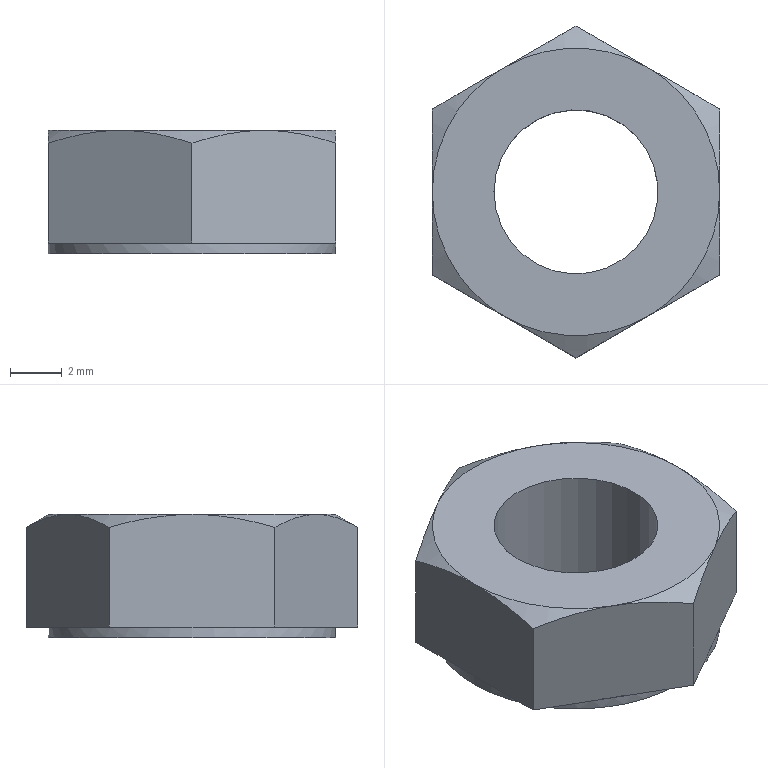Part | NX | features solid 2 | 1 solid | 22 faces | box 11.125 x 12.846 x 4.763 mm | volume 354.079 mm3 | plane 14 | cone 6 | cylinder 2 | commonest cylinder face diameters 6.35 x1 11.125 x1
STEP:
#1=CARTESIAN_POINT('',(2.781,4.817,4.763));
#2=VERTEX_POINT('',#1);
#3=CARTESIAN_POINT('',(0.,6.423,4.266));
#4=VERTEX_POINT('',#3);
#5=CARTESIAN_POINT('',(2.781,4.817,4.763));
#6=CARTESIAN_POINT('',(1.837,5.362,4.763));
#7=CARTESIAN_POINT('',(0.9077,5.899,4.568));
#8=CARTESIAN_POINT('',(0.,6.423,4.266));
#9=B_SPLINE_CURVE_WITH_KNOTS('',3,(#5,#6,#7,#8),.UNSPECIFIED.,.F.,.F.,(4,4),(0.00325,0.006487),.UNSPECIFIED.);
#10=EDGE_CURVE('',#2,#4,#9,.T.);
#11=ORIENTED_EDGE('',*,*,#10,.T.);
#12=CARTESIAN_POINT('',(-2.781,4.817,4.763));
#13=VERTEX_POINT('',#12);
#14=CARTESIAN_POINT('',(0.,6.423,4.266));
#15=CARTESIAN_POINT('',(-0.91,5.898,4.569));
#16=CARTESIAN_POINT('',(-1.834,5.365,4.763));
#17=CARTESIAN_POINT('',(-2.781,4.817,4.763));
#18=B_SPLINE_CURVE_WITH_KNOTS('',3,(#14,#15,#16,#17),.UNSPECIFIED.,.F.,.F.,(4,4),(0.000000238,0.00325),.UNSPECIFIED.);
#19=EDGE_CURVE('',#4,#13,#18,.T.);
#20=ORIENTED_EDGE('',*,*,#19,.T.);
#21=CARTESIAN_POINT('',(0.,0.,4.763));
#22=DIRECTION('',(0.,0.,-1.));
#23=DIRECTION('',(-1.,0.,0.));
#24=AXIS2_PLACEMENT_3D('',#21,#22,#23);
#25=CIRCLE('',#24,5.563);
#26=EDGE_CURVE('',#13,#2,#25,.T.);
#27=ORIENTED_EDGE('',*,*,#26,.T.);
#28=EDGE_LOOP('',(#11,#20,#27));
#29=FACE_BOUND('',#28,.T.);
#30=CARTESIAN_POINT('',(0.,0.,4.763));
#31=DIRECTION('',(0.,0.,-1.));
#32=DIRECTION('',(-1.,0.,0.));
#33=AXIS2_PLACEMENT_3D('',#30,#31,#32);
#34=CONICAL_SURFACE('',#33,5.563,1.047);
#35=ADVANCED_FACE('',(#29),#34,.T.);
#36=CARTESIAN_POINT('',(-5.563,0.,4.763));
#37=VERTEX_POINT('',#36);
#38=CARTESIAN_POINT('',(0.,0.,4.763));
#39=DIRECTION('',(0.,0.,-1.));
#40=DIRECTION('',(-1.,0.,0.));
#41=AXIS2_PLACEMENT_3D('',#38,#39,#40);
#42=CIRCLE('',#41,5.563);
#43=EDGE_CURVE('',#37,#13,#42,.T.);
#44=ORIENTED_EDGE('',*,*,#43,.T.);
#45=CARTESIAN_POINT('',(-5.563,3.212,4.266));
#46=VERTEX_POINT('',#45);
#47=CARTESIAN_POINT('',(-2.781,4.817,4.763));
#48=CARTESIAN_POINT('',(-3.725,4.272,4.763));
#49=CARTESIAN_POINT('',(-4.655,3.736,4.568));
#50=CARTESIAN_POINT('',(-5.563,3.212,4.266));
#51=B_SPLINE_CURVE_WITH_KNOTS('',3,(#47,#48,#49,#50),.UNSPECIFIED.,.F.,.F.,(4,4),(0.00325,0.006487),.UNSPECIFIED.);
#52=EDGE_CURVE('',#13,#46,#51,.T.);
#53=ORIENTED_EDGE('',*,*,#52,.T.);
#54=CARTESIAN_POINT('',(-5.563,0.,4.763));
#55=CARTESIAN_POINT('',(-5.563,1.087,4.763));
#56=CARTESIAN_POINT('',(-5.563,2.173,4.566));
#57=CARTESIAN_POINT('',(-5.563,3.212,4.266));
#58=B_SPLINE_CURVE_WITH_KNOTS('',3,(#54,#55,#56,#57),.UNSPECIFIED.,.F.,.F.,(4,4),(0.009152,0.01241),.UNSPECIFIED.);
#59=EDGE_CURVE('',#46,#37,#58,.F.);
#60=ORIENTED_EDGE('',*,*,#59,.T.);
#61=EDGE_LOOP('',(#44,#53,#60));
#62=FACE_BOUND('',#61,.T.);
#63=CARTESIAN_POINT('',(0.,0.,4.763));
#64=DIRECTION('',(0.,0.,-1.));
#65=DIRECTION('',(-1.,0.,0.));
#66=AXIS2_PLACEMENT_3D('',#63,#64,#65);
#67=CONICAL_SURFACE('',#66,5.563,1.047);
#68=ADVANCED_FACE('',(#62),#67,.T.);
#69=CARTESIAN_POINT('',(-2.781,-4.817,4.763));
#70=VERTEX_POINT('',#69);
#71=CARTESIAN_POINT('',(0.,0.,4.763));
#72=DIRECTION('',(0.,0.,-1.));
#73=DIRECTION('',(-1.,0.,0.));
#74=AXIS2_PLACEMENT_3D('',#71,#72,#73);
#75=CIRCLE('',#74,5.563);
#76=EDGE_CURVE('',#70,#37,#75,.T.);
#77=ORIENTED_EDGE('',*,*,#76,.T.);
#78=CARTESIAN_POINT('',(-5.563,-3.212,4.266));
#79=VERTEX_POINT('',#78);
#80=CARTESIAN_POINT('',(-5.563,-3.212,4.266));
#81=CARTESIAN_POINT('',(-5.563,-2.166,4.568));
#82=CARTESIAN_POINT('',(-5.563,-1.086,4.763));
#83=CARTESIAN_POINT('',(-5.563,0.,4.763));
#84=B_SPLINE_CURVE_WITH_KNOTS('',3,(#80,#81,#82,#83),.UNSPECIFIED.,.F.,.F.,(4,4),(0.005902,0.009152),.UNSPECIFIED.);
#85=EDGE_CURVE('',#37,#79,#84,.F.);
#86=ORIENTED_EDGE('',*,*,#85,.T.);
#87=CARTESIAN_POINT('',(-5.563,-3.212,4.266));
#88=CARTESIAN_POINT('',(-4.653,-3.737,4.569));
#89=CARTESIAN_POINT('',(-3.729,-4.27,4.763));
#90=CARTESIAN_POINT('',(-2.781,-4.817,4.763));
#91=B_SPLINE_CURVE_WITH_KNOTS('',3,(#87,#88,#89,#90),.UNSPECIFIED.,.F.,.F.,(4,4),(0.000000238,0.00325),.UNSPECIFIED.);
#92=EDGE_CURVE('',#79,#70,#91,.T.);
#93=ORIENTED_EDGE('',*,*,#92,.T.);
#94=EDGE_LOOP('',(#77,#86,#93));
#95=FACE_BOUND('',#94,.T.);
#96=CARTESIAN_POINT('',(0.,0.,4.763));
#97=DIRECTION('',(0.,0.,-1.));
#98=DIRECTION('',(-1.,0.,0.));
#99=AXIS2_PLACEMENT_3D('',#96,#97,#98);
#100=CONICAL_SURFACE('',#99,5.563,1.047);
#101=ADVANCED_FACE('',(#95),#100,.T.);
#102=CARTESIAN_POINT('',(2.781,-4.817,4.763));
#103=VERTEX_POINT('',#102);
#104=CARTESIAN_POINT('',(0.,0.,4.763));
#105=DIRECTION('',(0.,0.,-1.));
#106=DIRECTION('',(-1.,0.,0.));
#107=AXIS2_PLACEMENT_3D('',#104,#105,#106);
#108=CIRCLE('',#107,5.563);
#109=EDGE_CURVE('',#103,#70,#108,.T.);
#110=ORIENTED_EDGE('',*,*,#109,.T.);
#111=CARTESIAN_POINT('',(0.,-6.423,4.266));
#112=VERTEX_POINT('',#111);
#113=CARTESIAN_POINT('',(-2.781,-4.817,4.763));
#114=CARTESIAN_POINT('',(-1.837,-5.362,4.763));
#115=CARTESIAN_POINT('',(-0.9077,-5.899,4.568));
#116=CARTESIAN_POINT('',(0.,-6.423,4.266));
#117=B_SPLINE_CURVE_WITH_KNOTS('',3,(#113,#114,#115,#116),.UNSPECIFIED.,.F.,.F.,(4,4),(0.00325,0.006487),.UNSPECIFIED.);
#118=EDGE_CURVE('',#70,#112,#117,.T.);
#119=ORIENTED_EDGE('',*,*,#118,.T.);
#120=CARTESIAN_POINT('',(0.,-6.423,4.266));
#121=CARTESIAN_POINT('',(0.91,-5.898,4.569));
#122=CARTESIAN_POINT('',(1.834,-5.365,4.763));
#123=CARTESIAN_POINT('',(2.781,-4.817,4.763));
#124=B_SPLINE_CURVE_WITH_KNOTS('',3,(#120,#121,#122,#123),.UNSPECIFIED.,.F.,.F.,(4,4),(0.000000238,0.00325),.UNSPECIFIED.);
#125=EDGE_CURVE('',#112,#103,#124,.T.);
#126=ORIENTED_EDGE('',*,*,#125,.T.);
#127=EDGE_LOOP('',(#110,#119,#126));
#128=FACE_BOUND('',#127,.T.);
#129=CARTESIAN_POINT('',(0.,0.,4.763));
#130=DIRECTION('',(0.,0.,-1.));
#131=DIRECTION('',(-1.,0.,0.));
#132=AXIS2_PLACEMENT_3D('',#129,#130,#131);
#133=CONICAL_SURFACE('',#132,5.563,1.047);
#134=ADVANCED_FACE('',(#128),#133,.T.);
#135=CARTESIAN_POINT('',(5.563,0.,4.763));
#136=VERTEX_POINT('',#135);
#137=CARTESIAN_POINT('',(0.,0.,4.763));
#138=DIRECTION('',(0.,0.,-1.));
#139=DIRECTION('',(-1.,0.,0.));
#140=AXIS2_PLACEMENT_3D('',#137,#138,#139);
#141=CIRCLE('',#140,5.563);
#142=EDGE_CURVE('',#136,#103,#141,.T.);
#143=ORIENTED_EDGE('',*,*,#142,.T.);
#144=CARTESIAN_POINT('',(5.563,-3.212,4.266));
#145=VERTEX_POINT('',#144);
#146=CARTESIAN_POINT('',(2.781,-4.817,4.763));
#147=CARTESIAN_POINT('',(3.725,-4.272,4.763));
#148=CARTESIAN_POINT('',(4.655,-3.736,4.568));
#149=CARTESIAN_POINT('',(5.563,-3.212,4.266));
#150=B_SPLINE_CURVE_WITH_KNOTS('',3,(#146,#147,#148,#149),.UNSPECIFIED.,.F.,.F.,(4,4),(0.00325,0.006487),.UNSPECIFIED.);
#151=EDGE_CURVE('',#103,#145,#150,.T.);
#152=ORIENTED_EDGE('',*,*,#151,.T.);
#153=CARTESIAN_POINT('',(5.563,-3.212,4.266));
#154=CARTESIAN_POINT('',(5.563,-2.166,4.568));
#155=CARTESIAN_POINT('',(5.563,-1.086,4.763));
#156=CARTESIAN_POINT('',(5.563,0.,4.763));
#157=B_SPLINE_CURVE_WITH_KNOTS('',3,(#153,#154,#155,#156),.UNSPECIFIED.,.F.,.F.,(4,4),(0.005902,0.009152),.UNSPECIFIED.);
#158=EDGE_CURVE('',#145,#136,#157,.T.);
#159=ORIENTED_EDGE('',*,*,#158,.T.);
#160=EDGE_LOOP('',(#143,#152,#159));
#161=FACE_BOUND('',#160,.T.);
#162=CARTESIAN_POINT('',(0.,0.,4.763));
#163=DIRECTION('',(0.,0.,-1.));
#164=DIRECTION('',(-1.,0.,0.));
#165=AXIS2_PLACEMENT_3D('',#162,#163,#164);
#166=CONICAL_SURFACE('',#165,5.563,1.047);
#167=ADVANCED_FACE('',(#161),#166,.T.);
#168=CARTESIAN_POINT('',(0.,0.,4.763));
#169=DIRECTION('',(0.,0.,-1.));
#170=DIRECTION('',(-1.,0.,0.));
#171=AXIS2_PLACEMENT_3D('',#168,#169,#170);
#172=CIRCLE('',#171,5.563);
#173=EDGE_CURVE('',#2,#136,#172,.T.);
#174=ORIENTED_EDGE('',*,*,#173,.T.);
#175=CARTESIAN_POINT('',(5.563,3.212,4.266));
#176=VERTEX_POINT('',#175);
#177=CARTESIAN_POINT('',(5.563,0.,4.763));
#178=CARTESIAN_POINT('',(5.563,1.087,4.763));
#179=CARTESIAN_POINT('',(5.563,2.173,4.566));
#180=CARTESIAN_POINT('',(5.563,3.212,4.266));
#181=B_SPLINE_CURVE_WITH_KNOTS('',3,(#177,#178,#179,#180),.UNSPECIFIED.,.F.,.F.,(4,4),(0.009152,0.01241),.UNSPECIFIED.);
#182=EDGE_CURVE('',#136,#176,#181,.T.);
#183=ORIENTED_EDGE('',*,*,#182,.T.);
#184=CARTESIAN_POINT('',(5.563,3.212,4.266));
#185=CARTESIAN_POINT('',(4.653,3.737,4.569));
#186=CARTESIAN_POINT('',(3.729,4.27,4.763));
#187=CARTESIAN_POINT('',(2.781,4.817,4.763));
#188=B_SPLINE_CURVE_WITH_KNOTS('',3,(#184,#185,#186,#187),.UNSPECIFIED.,.F.,.F.,(4,4),(0.000000238,0.00325),.UNSPECIFIED.);
#189=EDGE_CURVE('',#176,#2,#188,.T.);
#190=ORIENTED_EDGE('',*,*,#189,.T.);
#191=EDGE_LOOP('',(#174,#183,#190));
#192=FACE_BOUND('',#191,.T.);
#193=CARTESIAN_POINT('',(0.,0.,4.763));
#194=DIRECTION('',(0.,0.,-1.));
#195=DIRECTION('',(-1.,0.,0.));
#196=AXIS2_PLACEMENT_3D('',#193,#194,#195);
#197=CONICAL_SURFACE('',#196,5.563,1.047);
#198=ADVANCED_FACE('',(#192),#197,.T.);
#199=CARTESIAN_POINT('',(2.781,-4.817,0.4064));
#200=VERTEX_POINT('',#199);
#201=CARTESIAN_POINT('',(0.,-6.423,0.4064));
#202=VERTEX_POINT('',#201);
#203=CARTESIAN_POINT('',(9.039,-1.204,0.4064));
#204=DIRECTION('',(-0.866,-0.5,0.));
#205=VECTOR('',#204,1000.);
#206=LINE('',#203,#205);
#207=EDGE_CURVE('',#200,#202,#206,.T.);
#208=ORIENTED_EDGE('',*,*,#207,.T.);
#209=CARTESIAN_POINT('',(-2.781,-4.817,0.4064));
#210=VERTEX_POINT('',#209);
#211=CARTESIAN_POINT('',(3.477,-8.43,0.4064));
#212=DIRECTION('',(-0.866,0.5,0.));
#213=VECTOR('',#212,1000.);
#214=LINE('',#211,#213);
#215=EDGE_CURVE('',#202,#210,#214,.T.);
#216=ORIENTED_EDGE('',*,*,#215,.T.);
#217=CARTESIAN_POINT('',(0.,0.,0.4064));
#218=DIRECTION('',(0.,0.,-1.));
#219=DIRECTION('',(-1.,0.,0.));
#220=AXIS2_PLACEMENT_3D('',#217,#218,#219);
#221=CIRCLE('',#220,5.563);
#222=EDGE_CURVE('',#200,#210,#221,.T.);
#223=ORIENTED_EDGE('',*,*,#222,.F.);
#224=EDGE_LOOP('',(#208,#216,#223));
#225=FACE_BOUND('',#224,.T.);
#226=CARTESIAN_POINT('',(8.344,0.,0.4064));
#227=DIRECTION('',(0.,0.,1.));
#228=DIRECTION('',(1.,0.,0.));
#229=AXIS2_PLACEMENT_3D('',#226,#227,#228);
#230=PLANE('',#229);
#231=ADVANCED_FACE('',(#225),#230,.F.);
#232=CARTESIAN_POINT('',(-5.563,0.,0.4064));
#233=VERTEX_POINT('',#232);
#234=CARTESIAN_POINT('',(0.,0.,0.4064));
#235=DIRECTION('',(0.,0.,-1.));
#236=DIRECTION('',(-1.,0.,0.));
#237=AXIS2_PLACEMENT_3D('',#234,#235,#236);
#238=CIRCLE('',#237,5.563);
#239=EDGE_CURVE('',#210,#233,#238,.T.);
#240=ORIENTED_EDGE('',*,*,#239,.F.);
#241=CARTESIAN_POINT('',(-5.563,-3.212,0.4064));
#242=VERTEX_POINT('',#241);
#243=CARTESIAN_POINT('',(3.477,-8.43,0.4064));
#244=DIRECTION('',(-0.866,0.5,0.));
#245=VECTOR('',#244,1000.);
#246=LINE('',#243,#245);
#247=EDGE_CURVE('',#210,#242,#246,.T.);
#248=ORIENTED_EDGE('',*,*,#247,.T.);
#249=CARTESIAN_POINT('',(-5.563,0.,0.4064));
#250=DIRECTION('',(0.,1.,0.));
#251=VECTOR('',#250,1000.);
#252=LINE('',#249,#251);
#253=EDGE_CURVE('',#242,#233,#252,.T.);
#254=ORIENTED_EDGE('',*,*,#253,.T.);
#255=EDGE_LOOP('',(#240,#248,#254));
#256=FACE_BOUND('',#255,.T.);
#257=CARTESIAN_POINT('',(8.344,0.,0.4064));
#258=DIRECTION('',(0.,0.,1.));
#259=DIRECTION('',(1.,0.,0.));
#260=AXIS2_PLACEMENT_3D('',#257,#258,#259);
#261=PLANE('',#260);
#262=ADVANCED_FACE('',(#256),#261,.F.);
#263=CARTESIAN_POINT('',(-2.781,4.817,0.4064));
#264=VERTEX_POINT('',#263);
#265=CARTESIAN_POINT('',(0.,0.,0.4064));
#266=DIRECTION('',(0.,0.,-1.));
#267=DIRECTION('',(-1.,0.,0.));
#268=AXIS2_PLACEMENT_3D('',#265,#266,#267);
#269=CIRCLE('',#268,5.563);
#270=EDGE_CURVE('',#233,#264,#269,.T.);
#271=ORIENTED_EDGE('',*,*,#270,.F.);
#272=CARTESIAN_POINT('',(-5.563,3.212,0.4064));
#273=VERTEX_POINT('',#272);
#274=CARTESIAN_POINT('',(-5.563,0.,0.4064));
#275=DIRECTION('',(0.,1.,0.));
#276=VECTOR('',#275,1000.);
#277=LINE('',#274,#276);
#278=EDGE_CURVE('',#233,#273,#277,.T.);
#279=ORIENTED_EDGE('',*,*,#278,.T.);
#280=CARTESIAN_POINT('',(3.477,8.43,0.4064));
#281=DIRECTION('',(0.866,0.5,0.));
#282=VECTOR('',#281,1000.);
#283=LINE('',#280,#282);
#284=EDGE_CURVE('',#273,#264,#283,.T.);
#285=ORIENTED_EDGE('',*,*,#284,.T.);
#286=EDGE_LOOP('',(#271,#279,#285));
#287=FACE_BOUND('',#286,.T.);
#288=CARTESIAN_POINT('',(8.344,0.,0.4064));
#289=DIRECTION('',(0.,0.,1.));
#290=DIRECTION('',(1.,0.,0.));
#291=AXIS2_PLACEMENT_3D('',#288,#289,#290);
#292=PLANE('',#291);
#293=ADVANCED_FACE('',(#287),#292,.F.);
#294=CARTESIAN_POINT('',(5.563,0.,0.4064));
#295=VERTEX_POINT('',#294);
#296=CARTESIAN_POINT('',(5.563,-3.212,0.4064));
#297=VERTEX_POINT('',#296);
#298=CARTESIAN_POINT('',(5.563,0.,0.4064));
#299=DIRECTION('',(0.,-1.,0.));
#300=VECTOR('',#299,1000.);
#301=LINE('',#298,#300);
#302=EDGE_CURVE('',#295,#297,#301,.T.);
#303=ORIENTED_EDGE('',*,*,#302,.T.);
#304=CARTESIAN_POINT('',(9.039,-1.204,0.4064));
#305=DIRECTION('',(-0.866,-0.5,0.));
#306=VECTOR('',#305,1000.);
#307=LINE('',#304,#306);
#308=EDGE_CURVE('',#297,#200,#307,.T.);
#309=ORIENTED_EDGE('',*,*,#308,.T.);
#310=CARTESIAN_POINT('',(0.,0.,0.4064));
#311=DIRECTION('',(0.,0.,-1.));
#312=DIRECTION('',(-1.,0.,0.));
#313=AXIS2_PLACEMENT_3D('',#310,#311,#312);
#314=CIRCLE('',#313,5.563);
#315=EDGE_CURVE('',#295,#200,#314,.T.);
#316=ORIENTED_EDGE('',*,*,#315,.F.);
#317=EDGE_LOOP('',(#303,#309,#316));
#318=FACE_BOUND('',#317,.T.);
#319=CARTESIAN_POINT('',(8.344,0.,0.4064));
#320=DIRECTION('',(0.,0.,1.));
#321=DIRECTION('',(1.,0.,0.));
#322=AXIS2_PLACEMENT_3D('',#319,#320,#321);
#323=PLANE('',#322);
#324=ADVANCED_FACE('',(#318),#323,.F.);
#325=CARTESIAN_POINT('',(2.781,4.817,0.4064));
#326=VERTEX_POINT('',#325);
#327=CARTESIAN_POINT('',(0.,0.,0.4064));
#328=DIRECTION('',(0.,0.,-1.));
#329=DIRECTION('',(-1.,0.,0.));
#330=AXIS2_PLACEMENT_3D('',#327,#328,#329);
#331=CIRCLE('',#330,5.563);
#332=EDGE_CURVE('',#264,#326,#331,.T.);
#333=ORIENTED_EDGE('',*,*,#332,.F.);
#334=CARTESIAN_POINT('',(0.,6.423,0.4064));
#335=VERTEX_POINT('',#334);
#336=CARTESIAN_POINT('',(3.477,8.43,0.4064));
#337=DIRECTION('',(0.866,0.5,0.));
#338=VECTOR('',#337,1000.);
#339=LINE('',#336,#338);
#340=EDGE_CURVE('',#264,#335,#339,.T.);
#341=ORIENTED_EDGE('',*,*,#340,.T.);
#342=CARTESIAN_POINT('',(9.039,1.204,0.4064));
#343=DIRECTION('',(0.866,-0.5,0.));
#344=VECTOR('',#343,1000.);
#345=LINE('',#342,#344);
#346=EDGE_CURVE('',#335,#326,#345,.T.);
#347=ORIENTED_EDGE('',*,*,#346,.T.);
#348=EDGE_LOOP('',(#333,#341,#347));
#349=FACE_BOUND('',#348,.T.);
#350=CARTESIAN_POINT('',(8.344,0.,0.4064));
#351=DIRECTION('',(0.,0.,1.));
#352=DIRECTION('',(1.,0.,0.));
#353=AXIS2_PLACEMENT_3D('',#350,#351,#352);
#354=PLANE('',#353);
#355=ADVANCED_FACE('',(#349),#354,.F.);
#356=CARTESIAN_POINT('',(5.563,3.212,0.4064));
#357=VERTEX_POINT('',#356);
#358=CARTESIAN_POINT('',(9.039,1.204,0.4064));
#359=DIRECTION('',(0.866,-0.5,0.));
#360=VECTOR('',#359,1000.);
#361=LINE('',#358,#360);
#362=EDGE_CURVE('',#326,#357,#361,.T.);
#363=ORIENTED_EDGE('',*,*,#362,.T.);
#364=CARTESIAN_POINT('',(5.563,0.,0.4064));
#365=DIRECTION('',(0.,-1.,0.));
#366=VECTOR('',#365,1000.);
#367=LINE('',#364,#366);
#368=EDGE_CURVE('',#357,#295,#367,.T.);
#369=ORIENTED_EDGE('',*,*,#368,.T.);
#370=CARTESIAN_POINT('',(0.,0.,0.4064));
#371=DIRECTION('',(0.,0.,-1.));
#372=DIRECTION('',(-1.,0.,0.));
#373=AXIS2_PLACEMENT_3D('',#370,#371,#372);
#374=CIRCLE('',#373,5.563);
#375=EDGE_CURVE('',#326,#295,#374,.T.);
#376=ORIENTED_EDGE('',*,*,#375,.F.);
#377=EDGE_LOOP('',(#363,#369,#376));
#378=FACE_BOUND('',#377,.T.);
#379=CARTESIAN_POINT('',(8.344,0.,0.4064));
#380=DIRECTION('',(0.,0.,1.));
#381=DIRECTION('',(1.,0.,0.));
#382=AXIS2_PLACEMENT_3D('',#379,#380,#381);
#383=PLANE('',#382);
#384=ADVANCED_FACE('',(#378),#383,.F.);
#385=ORIENTED_EDGE('',*,*,#43,.F.);
#386=ORIENTED_EDGE('',*,*,#76,.F.);
#387=ORIENTED_EDGE('',*,*,#109,.F.);
#388=ORIENTED_EDGE('',*,*,#142,.F.);
#389=ORIENTED_EDGE('',*,*,#173,.F.);
#390=ORIENTED_EDGE('',*,*,#26,.F.);
#391=EDGE_LOOP('',(#385,#386,#387,#388,#389,#390));
#392=FACE_BOUND('',#391,.T.);
#393=CARTESIAN_POINT('',(-3.175,0.,4.763));
#394=VERTEX_POINT('',#393);
#395=CARTESIAN_POINT('',(0.,0.,4.763));
#396=DIRECTION('',(0.,0.,-1.));
#397=DIRECTION('',(-1.,0.,0.));
#398=AXIS2_PLACEMENT_3D('',#395,#396,#397);
#399=CIRCLE('',#398,3.175);
#400=EDGE_CURVE('',#394,#394,#399,.T.);
#401=ORIENTED_EDGE('',*,*,#400,.T.);
#402=EDGE_LOOP('',(#401));
#403=FACE_BOUND('',#402,.T.);
#404=CARTESIAN_POINT('',(3.175,0.,4.763));
#405=DIRECTION('',(0.,0.,-1.));
#406=DIRECTION('',(-1.,0.,0.));
#407=AXIS2_PLACEMENT_3D('',#404,#405,#406);
#408=PLANE('',#407);
#409=ADVANCED_FACE('',(#392,#403),#408,.F.);
#410=CARTESIAN_POINT('',(-5.563,0.,0.));
#411=VERTEX_POINT('',#410);
#412=CARTESIAN_POINT('',(0.,0.,0.));
#413=DIRECTION('',(0.,0.,-1.));
#414=DIRECTION('',(-1.,0.,0.));
#415=AXIS2_PLACEMENT_3D('',#412,#413,#414);
#416=CIRCLE('',#415,5.563);
#417=EDGE_CURVE('',#411,#411,#416,.T.);
#418=ORIENTED_EDGE('',*,*,#417,.F.);
#419=EDGE_LOOP('',(#418));
#420=FACE_BOUND('',#419,.T.);
#421=ORIENTED_EDGE('',*,*,#270,.T.);
#422=ORIENTED_EDGE('',*,*,#332,.T.);
#423=ORIENTED_EDGE('',*,*,#375,.T.);
#424=ORIENTED_EDGE('',*,*,#315,.T.);
#425=ORIENTED_EDGE('',*,*,#222,.T.);
#426=ORIENTED_EDGE('',*,*,#239,.T.);
#427=EDGE_LOOP('',(#421,#422,#423,#424,#425,#426));
#428=FACE_BOUND('',#427,.T.);
#429=CARTESIAN_POINT('',(0.,0.,0.));
#430=DIRECTION('',(0.,0.,-1.));
#431=DIRECTION('',(-1.,0.,0.));
#432=AXIS2_PLACEMENT_3D('',#429,#430,#431);
#433=CYLINDRICAL_SURFACE('',#432,5.563);
#434=ADVANCED_FACE('',(#420,#428),#433,.T.);
#435=CARTESIAN_POINT('',(-3.175,0.,0.));
#436=VERTEX_POINT('',#435);
#437=CARTESIAN_POINT('',(0.,0.,0.));
#438=DIRECTION('',(0.,0.,-1.));
#439=DIRECTION('',(-1.,0.,0.));
#440=AXIS2_PLACEMENT_3D('',#437,#438,#439);
#441=CIRCLE('',#440,3.175);
#442=EDGE_CURVE('',#436,#436,#441,.T.);
#443=ORIENTED_EDGE('',*,*,#442,.F.);
#444=EDGE_LOOP('',(#443));
#445=FACE_BOUND('',#444,.T.);
#446=ORIENTED_EDGE('',*,*,#417,.T.);
#447=EDGE_LOOP('',(#446));
#448=FACE_BOUND('',#447,.T.);
#449=CARTESIAN_POINT('',(5.563,0.,0.));
#450=DIRECTION('',(0.,0.,1.));
#451=DIRECTION('',(1.,0.,0.));
#452=AXIS2_PLACEMENT_3D('',#449,#450,#451);
#453=PLANE('',#452);
#454=ADVANCED_FACE('',(#445,#448),#453,.F.);
#455=ORIENTED_EDGE('',*,*,#400,.F.);
#456=EDGE_LOOP('',(#455));
#457=FACE_BOUND('',#456,.T.);
#458=ORIENTED_EDGE('',*,*,#442,.T.);
#459=EDGE_LOOP('',(#458));
#460=FACE_BOUND('',#459,.T.);
#461=CARTESIAN_POINT('',(0.,0.,0.));
#462=DIRECTION('',(0.,0.,-1.));
#463=DIRECTION('',(-1.,0.,0.));
#464=AXIS2_PLACEMENT_3D('',#461,#462,#463);
#465=CYLINDRICAL_SURFACE('',#464,3.175);
#466=ADVANCED_FACE('',(#457,#460),#465,.F.);
#467=ORIENTED_EDGE('',*,*,#19,.F.);
#468=CARTESIAN_POINT('',(0.,6.423,5.239));
#469=DIRECTION('',(0.,0.,-1.));
#470=VECTOR('',#469,1000.);
#471=LINE('',#468,#470);
#472=EDGE_CURVE('',#4,#335,#471,.T.);
#473=ORIENTED_EDGE('',*,*,#472,.T.);
#474=ORIENTED_EDGE('',*,*,#340,.F.);
#475=ORIENTED_EDGE('',*,*,#284,.F.);
#476=CARTESIAN_POINT('',(-5.563,3.212,5.239));
#477=DIRECTION('',(0.,0.,-1.));
#478=VECTOR('',#477,1000.);
#479=LINE('',#476,#478);
#480=EDGE_CURVE('',#46,#273,#479,.T.);
#481=ORIENTED_EDGE('',*,*,#480,.F.);
#482=ORIENTED_EDGE('',*,*,#52,.F.);
#483=EDGE_LOOP('',(#467,#473,#474,#475,#481,#482));
#484=FACE_BOUND('',#483,.T.);
#485=CARTESIAN_POINT('',(0.,6.423,5.239));
#486=DIRECTION('',(0.5,-0.866,0.));
#487=DIRECTION('',(0.866,0.5,0.));
#488=AXIS2_PLACEMENT_3D('',#485,#486,#487);
#489=PLANE('',#488);
#490=ADVANCED_FACE('',(#484),#489,.F.);
#491=ORIENTED_EDGE('',*,*,#59,.F.);
#492=ORIENTED_EDGE('',*,*,#480,.T.);
#493=ORIENTED_EDGE('',*,*,#278,.F.);
#494=ORIENTED_EDGE('',*,*,#253,.F.);
#495=CARTESIAN_POINT('',(-5.563,-3.212,5.239));
#496=DIRECTION('',(0.,0.,-1.));
#497=VECTOR('',#496,1000.);
#498=LINE('',#495,#497);
#499=EDGE_CURVE('',#79,#242,#498,.T.);
#500=ORIENTED_EDGE('',*,*,#499,.F.);
#501=ORIENTED_EDGE('',*,*,#85,.F.);
#502=EDGE_LOOP('',(#491,#492,#493,#494,#500,#501));
#503=FACE_BOUND('',#502,.T.);
#504=CARTESIAN_POINT('',(-5.563,3.212,5.239));
#505=DIRECTION('',(1.,0.,0.));
#506=DIRECTION('',(0.,1.,0.));
#507=AXIS2_PLACEMENT_3D('',#504,#505,#506);
#508=PLANE('',#507);
#509=ADVANCED_FACE('',(#503),#508,.F.);
#510=ORIENTED_EDGE('',*,*,#92,.F.);
#511=ORIENTED_EDGE('',*,*,#499,.T.);
#512=ORIENTED_EDGE('',*,*,#247,.F.);
#513=ORIENTED_EDGE('',*,*,#215,.F.);
#514=CARTESIAN_POINT('',(0.,-6.423,5.239));
#515=DIRECTION('',(0.,0.,-1.));
#516=VECTOR('',#515,1000.);
#517=LINE('',#514,#516);
#518=EDGE_CURVE('',#112,#202,#517,.T.);
#519=ORIENTED_EDGE('',*,*,#518,.F.);
#520=ORIENTED_EDGE('',*,*,#118,.F.);
#521=EDGE_LOOP('',(#510,#511,#512,#513,#519,#520));
#522=FACE_BOUND('',#521,.T.);
#523=CARTESIAN_POINT('',(-5.563,-3.212,5.239));
#524=DIRECTION('',(0.5,0.866,0.));
#525=DIRECTION('',(-0.866,0.5,0.));
#526=AXIS2_PLACEMENT_3D('',#523,#524,#525);
#527=PLANE('',#526);
#528=ADVANCED_FACE('',(#522),#527,.F.);
#529=ORIENTED_EDGE('',*,*,#125,.F.);
#530=ORIENTED_EDGE('',*,*,#518,.T.);
#531=ORIENTED_EDGE('',*,*,#207,.F.);
#532=ORIENTED_EDGE('',*,*,#308,.F.);
#533=CARTESIAN_POINT('',(5.563,-3.212,5.239));
#534=DIRECTION('',(0.,0.,-1.));
#535=VECTOR('',#534,1000.);
#536=LINE('',#533,#535);
#537=EDGE_CURVE('',#145,#297,#536,.T.);
#538=ORIENTED_EDGE('',*,*,#537,.F.);
#539=ORIENTED_EDGE('',*,*,#151,.F.);
#540=EDGE_LOOP('',(#529,#530,#531,#532,#538,#539));
#541=FACE_BOUND('',#540,.T.);
#542=CARTESIAN_POINT('',(0.,-6.423,5.239));
#543=DIRECTION('',(-0.5,0.866,0.));
#544=DIRECTION('',(-0.866,-0.5,0.));
#545=AXIS2_PLACEMENT_3D('',#542,#543,#544);
#546=PLANE('',#545);
#547=ADVANCED_FACE('',(#541),#546,.F.);
#548=ORIENTED_EDGE('',*,*,#158,.F.);
#549=ORIENTED_EDGE('',*,*,#537,.T.);
#550=ORIENTED_EDGE('',*,*,#302,.F.);
#551=ORIENTED_EDGE('',*,*,#368,.F.);
#552=CARTESIAN_POINT('',(5.563,3.212,5.239));
#553=DIRECTION('',(0.,0.,-1.));
#554=VECTOR('',#553,1000.);
#555=LINE('',#552,#554);
#556=EDGE_CURVE('',#176,#357,#555,.T.);
#557=ORIENTED_EDGE('',*,*,#556,.F.);
#558=ORIENTED_EDGE('',*,*,#182,.F.);
#559=EDGE_LOOP('',(#548,#549,#550,#551,#557,#558));
#560=FACE_BOUND('',#559,.T.);
#561=CARTESIAN_POINT('',(5.563,-3.212,5.239));
#562=DIRECTION('',(-1.,0.,0.));
#563=DIRECTION('',(0.,-1.,0.));
#564=AXIS2_PLACEMENT_3D('',#561,#562,#563);
#565=PLANE('',#564);
#566=ADVANCED_FACE('',(#560),#565,.F.);
#567=ORIENTED_EDGE('',*,*,#189,.F.);
#568=ORIENTED_EDGE('',*,*,#556,.T.);
#569=ORIENTED_EDGE('',*,*,#362,.F.);
#570=ORIENTED_EDGE('',*,*,#346,.F.);
#571=ORIENTED_EDGE('',*,*,#472,.F.);
#572=ORIENTED_EDGE('',*,*,#10,.F.);
#573=EDGE_LOOP('',(#567,#568,#569,#570,#571,#572));
#574=FACE_BOUND('',#573,.T.);
#575=CARTESIAN_POINT('',(5.563,3.212,5.239));
#576=DIRECTION('',(-0.5,-0.866,0.));
#577=DIRECTION('',(0.866,-0.5,0.));
#578=AXIS2_PLACEMENT_3D('',#575,#576,#577);
#579=PLANE('',#578);
#580=ADVANCED_FACE('',(#574),#579,.F.);
#581=CLOSED_SHELL('',(#35,#68,#101,#134,#167,#198,#231,#262,#293,#324,#355,#384,#409,#434,#454,#466,#490,#509,#528,#547,#566,#580));
#582=MANIFOLD_SOLID_BREP('',#581);
#583=(LENGTH_UNIT()NAMED_UNIT(*)SI_UNIT(.MILLI.,.METRE.));
#584=UNCERTAINTY_MEASURE_WITH_UNIT(LENGTH_MEASURE(0.0508),#583,'','');
#585=(NAMED_UNIT(*)PLANE_ANGLE_UNIT()SI_UNIT($,.RADIAN.));
#586=(NAMED_UNIT(*)SI_UNIT($,.STERADIAN.)SOLID_ANGLE_UNIT());
#587=(GEOMETRIC_REPRESENTATION_CONTEXT(3)GLOBAL_UNCERTAINTY_ASSIGNED_CONTEXT((#584))GLOBAL_UNIT_ASSIGNED_CONTEXT((#583,#585,#586))REPRESENTATION_CONTEXT('',''));
#588=ADVANCED_BREP_SHAPE_REPRESENTATION('',(#582),#587);